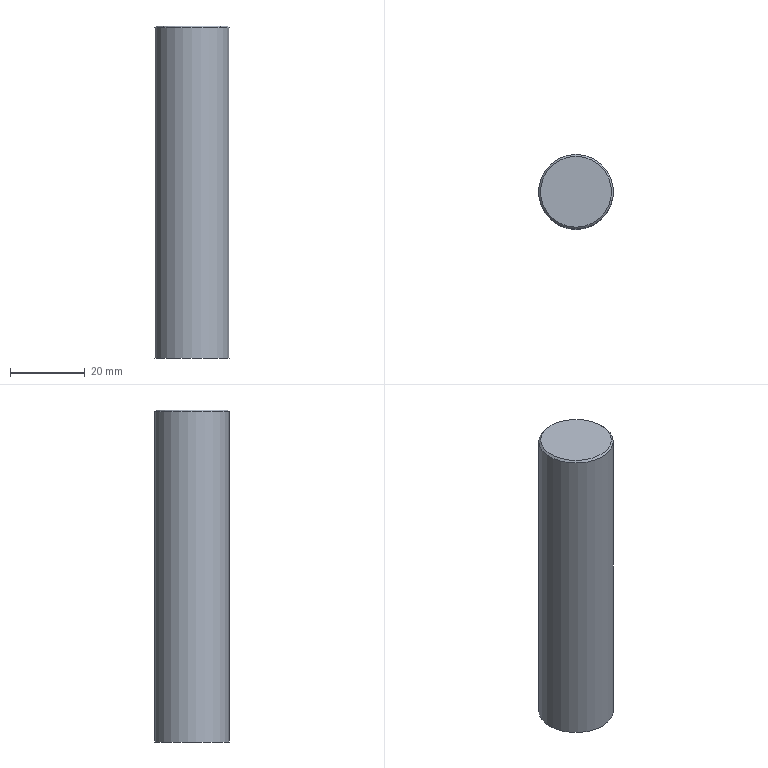Part | NX | features solid 2 | 1 solid | 4 faces | box 20 x 20 x 89 mm | volume 27952 mm3 | plane 2 | cylinder 1 | cone 1 | commonest cylinder face diameters 20 x1
STEP:
#1=CARTESIAN_POINT('',(255.,-20.,14.5));
#2=VERTEX_POINT('',#1);
#3=CARTESIAN_POINT('',(255.,-10.,14.5));
#4=DIRECTION('',(0.,0.,-1.));
#5=DIRECTION('',(0.,-1.,0.));
#6=AXIS2_PLACEMENT_3D('',#3,#4,#5);
#7=CIRCLE('',#6,10.);
#8=EDGE_CURVE('',#2,#2,#7,.T.);
#9=ORIENTED_EDGE('',*,*,#8,.T.);
#10=EDGE_LOOP('',(#9));
#11=FACE_BOUND('',#10,.T.);
#12=CARTESIAN_POINT('',(255.,-20.,-74.));
#13=VERTEX_POINT('',#12);
#14=CARTESIAN_POINT('',(255.,-10.,-74.));
#15=DIRECTION('',(0.,0.,-1.));
#16=DIRECTION('',(0.,-1.,0.));
#17=AXIS2_PLACEMENT_3D('',#14,#15,#16);
#18=CIRCLE('',#17,10.);
#19=EDGE_CURVE('',#13,#13,#18,.T.);
#20=ORIENTED_EDGE('',*,*,#19,.F.);
#21=EDGE_LOOP('',(#20));
#22=FACE_BOUND('',#21,.T.);
#23=CARTESIAN_POINT('',(255.,-10.,-74.));
#24=DIRECTION('',(0.,0.,1.));
#25=DIRECTION('',(0.,1.,0.));
#26=AXIS2_PLACEMENT_3D('',#23,#24,#25);
#27=CYLINDRICAL_SURFACE('',#26,10.);
#28=ADVANCED_FACE('',(#11,#22),#27,.T.);
#29=ORIENTED_EDGE('',*,*,#19,.T.);
#30=EDGE_LOOP('',(#29));
#31=FACE_BOUND('',#30,.T.);
#32=CARTESIAN_POINT('',(255.,-10.,-74.));
#33=DIRECTION('',(0.,0.,-1.));
#34=DIRECTION('',(0.,-1.,0.));
#35=AXIS2_PLACEMENT_3D('',#32,#33,#34);
#36=PLANE('',#35);
#37=ADVANCED_FACE('',(#31),#36,.T.);
#38=CARTESIAN_POINT('',(255.,-19.5,15.));
#39=VERTEX_POINT('',#38);
#40=CARTESIAN_POINT('',(255.,-10.,15.));
#41=DIRECTION('',(0.,0.,-1.));
#42=DIRECTION('',(0.,-1.,0.));
#43=AXIS2_PLACEMENT_3D('',#40,#41,#42);
#44=CIRCLE('',#43,9.5);
#45=EDGE_CURVE('',#39,#39,#44,.F.);
#46=ORIENTED_EDGE('',*,*,#45,.T.);
#47=EDGE_LOOP('',(#46));
#48=FACE_BOUND('',#47,.T.);
#49=CARTESIAN_POINT('',(255.,-10.,15.));
#50=DIRECTION('',(0.,0.,-1.));
#51=DIRECTION('',(0.,-1.,0.));
#52=AXIS2_PLACEMENT_3D('',#49,#50,#51);
#53=PLANE('',#52);
#54=ADVANCED_FACE('',(#48),#53,.F.);
#55=ORIENTED_EDGE('',*,*,#45,.F.);
#56=EDGE_LOOP('',(#55));
#57=FACE_BOUND('',#56,.T.);
#58=ORIENTED_EDGE('',*,*,#8,.F.);
#59=EDGE_LOOP('',(#58));
#60=FACE_BOUND('',#59,.T.);
#61=CARTESIAN_POINT('',(255.,-10.,14.5));
#62=DIRECTION('',(0.,0.,-1.));
#63=DIRECTION('',(0.,-1.,0.));
#64=AXIS2_PLACEMENT_3D('',#61,#62,#63);
#65=CONICAL_SURFACE('',#64,10.,0.7854);
#66=ADVANCED_FACE('',(#57,#60),#65,.T.);
#67=CLOSED_SHELL('',(#28,#37,#54,#66));
#68=MANIFOLD_SOLID_BREP('',#67);
#69=(LENGTH_UNIT()NAMED_UNIT(*)SI_UNIT(.MILLI.,.METRE.));
#70=UNCERTAINTY_MEASURE_WITH_UNIT(LENGTH_MEASURE(0.00001),#69,'','');
#71=(NAMED_UNIT(*)PLANE_ANGLE_UNIT()SI_UNIT($,.RADIAN.));
#72=(NAMED_UNIT(*)SI_UNIT($,.STERADIAN.)SOLID_ANGLE_UNIT());
#73=(GEOMETRIC_REPRESENTATION_CONTEXT(3)GLOBAL_UNCERTAINTY_ASSIGNED_CONTEXT((#70))GLOBAL_UNIT_ASSIGNED_CONTEXT((#69,#71,#72))REPRESENTATION_CONTEXT('',''));
#74=ADVANCED_BREP_SHAPE_REPRESENTATION('',(#68),#73);